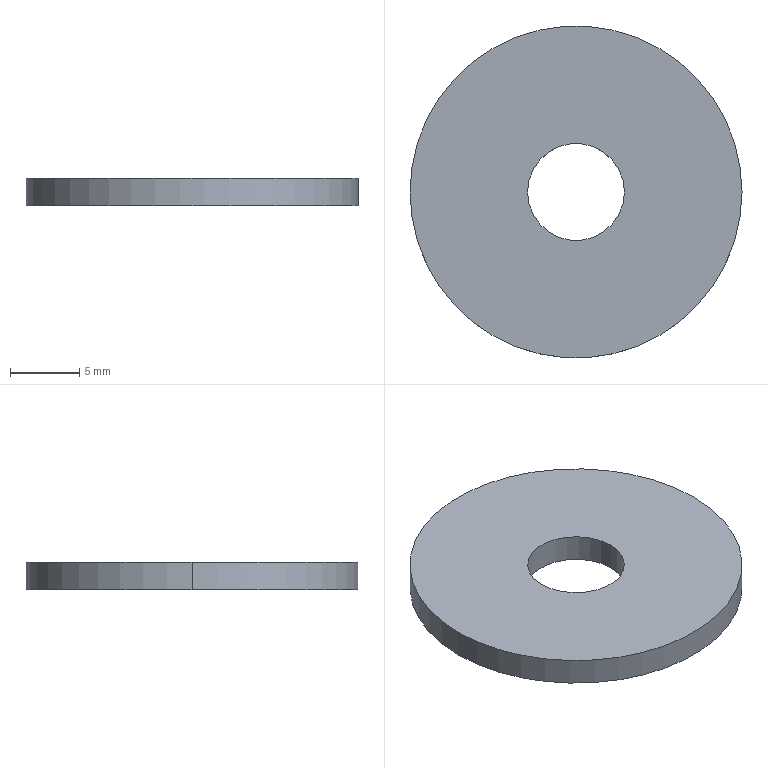Part | SolidWorks | features BaseBody 1 | 1 solid | 6 faces | box 24 x 24 x 2 mm | volume 827.81 mm3 | cylinder 4 | plane 2 | commonest cylinder face diameters 7 x2 24 x2
STEP:
#1=CARTESIAN_POINT('',(-12.,0.,2.));
#2=VERTEX_POINT('',#1);
#3=CARTESIAN_POINT('',(12.,0.,2.));
#4=VERTEX_POINT('',#3);
#5=CARTESIAN_POINT('',(0.,0.,2.));
#6=DIRECTION('',(0.,0.,-1.));
#7=DIRECTION('',(-1.,0.,0.));
#8=AXIS2_PLACEMENT_3D('',#5,#6,#7);
#9=CIRCLE('',#8,12.);
#10=EDGE_CURVE('',#2,#4,#9,.T.);
#11=ORIENTED_EDGE('',*,*,#10,.T.);
#12=CARTESIAN_POINT('',(12.,0.,0.));
#13=VERTEX_POINT('',#12);
#14=CARTESIAN_POINT('',(12.,0.,2.));
#15=DIRECTION('',(0.,0.,-1.));
#16=VECTOR('',#15,1000.);
#17=LINE('',#14,#16);
#18=EDGE_CURVE('',#4,#13,#17,.T.);
#19=ORIENTED_EDGE('',*,*,#18,.T.);
#20=CARTESIAN_POINT('',(-12.,0.,0.));
#21=VERTEX_POINT('',#20);
#22=CARTESIAN_POINT('',(0.,0.,0.));
#23=DIRECTION('',(0.,0.,1.));
#24=DIRECTION('',(-1.,0.,0.));
#25=AXIS2_PLACEMENT_3D('',#22,#23,#24);
#26=CIRCLE('',#25,12.);
#27=EDGE_CURVE('',#13,#21,#26,.T.);
#28=ORIENTED_EDGE('',*,*,#27,.T.);
#29=CARTESIAN_POINT('',(-12.,0.,2.));
#30=DIRECTION('',(0.,0.,-1.));
#31=VECTOR('',#30,1000.);
#32=LINE('',#29,#31);
#33=EDGE_CURVE('',#2,#21,#32,.T.);
#34=ORIENTED_EDGE('',*,*,#33,.F.);
#35=EDGE_LOOP('',(#11,#19,#28,#34));
#36=FACE_OUTER_BOUND('',#35,.T.);
#37=CARTESIAN_POINT('',(0.,0.,2.));
#38=DIRECTION('',(0.,0.,-1.));
#39=DIRECTION('',(-1.,0.,0.));
#40=AXIS2_PLACEMENT_3D('',#37,#38,#39);
#41=CYLINDRICAL_SURFACE('',#40,12.);
#42=ADVANCED_FACE('',(#36),#41,.T.);
#43=CARTESIAN_POINT('',(3.5,0.,0.));
#44=VERTEX_POINT('',#43);
#45=CARTESIAN_POINT('',(-3.5,0.,0.));
#46=VERTEX_POINT('',#45);
#47=CARTESIAN_POINT('',(0.,0.,0.));
#48=DIRECTION('',(0.,0.,-1.));
#49=DIRECTION('',(1.,0.,0.));
#50=AXIS2_PLACEMENT_3D('',#47,#48,#49);
#51=CIRCLE('',#50,3.5);
#52=EDGE_CURVE('',#44,#46,#51,.T.);
#53=ORIENTED_EDGE('',*,*,#52,.T.);
#54=CARTESIAN_POINT('',(-3.5,0.,2.));
#55=VERTEX_POINT('',#54);
#56=CARTESIAN_POINT('',(-3.5,0.,2.));
#57=DIRECTION('',(0.,0.,1.));
#58=VECTOR('',#57,1000.);
#59=LINE('',#56,#58);
#60=EDGE_CURVE('',#46,#55,#59,.T.);
#61=ORIENTED_EDGE('',*,*,#60,.T.);
#62=CARTESIAN_POINT('',(3.5,0.,2.));
#63=VERTEX_POINT('',#62);
#64=CARTESIAN_POINT('',(0.,0.,2.));
#65=DIRECTION('',(0.,0.,-1.));
#66=DIRECTION('',(1.,0.,0.));
#67=AXIS2_PLACEMENT_3D('',#64,#65,#66);
#68=CIRCLE('',#67,3.5);
#69=EDGE_CURVE('',#63,#55,#68,.T.);
#70=ORIENTED_EDGE('',*,*,#69,.F.);
#71=CARTESIAN_POINT('',(3.5,0.,2.));
#72=DIRECTION('',(0.,0.,1.));
#73=VECTOR('',#72,1000.);
#74=LINE('',#71,#73);
#75=EDGE_CURVE('',#44,#63,#74,.T.);
#76=ORIENTED_EDGE('',*,*,#75,.F.);
#77=EDGE_LOOP('',(#53,#61,#70,#76));
#78=FACE_OUTER_BOUND('',#77,.T.);
#79=CARTESIAN_POINT('',(0.,0.,2.));
#80=DIRECTION('',(0.,0.,1.));
#81=DIRECTION('',(1.,0.,0.));
#82=AXIS2_PLACEMENT_3D('',#79,#80,#81);
#83=CYLINDRICAL_SURFACE('',#82,3.5);
#84=ADVANCED_FACE('',(#78),#83,.F.);
#85=CARTESIAN_POINT('',(0.,0.,0.));
#86=DIRECTION('',(0.,0.,1.));
#87=DIRECTION('',(-1.,0.,0.));
#88=AXIS2_PLACEMENT_3D('',#85,#86,#87);
#89=CIRCLE('',#88,12.);
#90=EDGE_CURVE('',#21,#13,#89,.T.);
#91=ORIENTED_EDGE('',*,*,#90,.F.);
#92=ORIENTED_EDGE('',*,*,#27,.F.);
#93=EDGE_LOOP('',(#91,#92));
#94=FACE_OUTER_BOUND('',#93,.T.);
#95=ORIENTED_EDGE('',*,*,#52,.F.);
#96=CARTESIAN_POINT('',(0.,0.,0.));
#97=DIRECTION('',(0.,0.,-1.));
#98=DIRECTION('',(1.,0.,0.));
#99=AXIS2_PLACEMENT_3D('',#96,#97,#98);
#100=CIRCLE('',#99,3.5);
#101=EDGE_CURVE('',#46,#44,#100,.T.);
#102=ORIENTED_EDGE('',*,*,#101,.F.);
#103=EDGE_LOOP('',(#95,#102));
#104=FACE_BOUND('',#103,.T.);
#105=CARTESIAN_POINT('',(0.,0.,0.));
#106=DIRECTION('',(0.,0.,1.));
#107=DIRECTION('',(1.,0.,0.));
#108=AXIS2_PLACEMENT_3D('',#105,#106,#107);
#109=PLANE('',#108);
#110=ADVANCED_FACE('',(#94,#104),#109,.F.);
#111=ORIENTED_EDGE('',*,*,#18,.F.);
#112=CARTESIAN_POINT('',(0.,0.,2.));
#113=DIRECTION('',(0.,0.,-1.));
#114=DIRECTION('',(-1.,0.,0.));
#115=AXIS2_PLACEMENT_3D('',#112,#113,#114);
#116=CIRCLE('',#115,12.);
#117=EDGE_CURVE('',#4,#2,#116,.T.);
#118=ORIENTED_EDGE('',*,*,#117,.T.);
#119=ORIENTED_EDGE('',*,*,#33,.T.);
#120=ORIENTED_EDGE('',*,*,#90,.T.);
#121=EDGE_LOOP('',(#111,#118,#119,#120));
#122=FACE_OUTER_BOUND('',#121,.T.);
#123=CARTESIAN_POINT('',(0.,0.,2.));
#124=DIRECTION('',(0.,0.,-1.));
#125=DIRECTION('',(-1.,0.,0.));
#126=AXIS2_PLACEMENT_3D('',#123,#124,#125);
#127=CYLINDRICAL_SURFACE('',#126,12.);
#128=ADVANCED_FACE('',(#122),#127,.T.);
#129=ORIENTED_EDGE('',*,*,#60,.F.);
#130=ORIENTED_EDGE('',*,*,#101,.T.);
#131=ORIENTED_EDGE('',*,*,#75,.T.);
#132=CARTESIAN_POINT('',(0.,0.,2.));
#133=DIRECTION('',(0.,0.,-1.));
#134=DIRECTION('',(1.,0.,0.));
#135=AXIS2_PLACEMENT_3D('',#132,#133,#134);
#136=CIRCLE('',#135,3.5);
#137=EDGE_CURVE('',#55,#63,#136,.T.);
#138=ORIENTED_EDGE('',*,*,#137,.F.);
#139=EDGE_LOOP('',(#129,#130,#131,#138));
#140=FACE_OUTER_BOUND('',#139,.T.);
#141=CARTESIAN_POINT('',(0.,0.,2.));
#142=DIRECTION('',(0.,0.,1.));
#143=DIRECTION('',(1.,0.,0.));
#144=AXIS2_PLACEMENT_3D('',#141,#142,#143);
#145=CYLINDRICAL_SURFACE('',#144,3.5);
#146=ADVANCED_FACE('',(#140),#145,.F.);
#147=ORIENTED_EDGE('',*,*,#10,.F.);
#148=ORIENTED_EDGE('',*,*,#117,.F.);
#149=EDGE_LOOP('',(#147,#148));
#150=FACE_OUTER_BOUND('',#149,.T.);
#151=ORIENTED_EDGE('',*,*,#69,.T.);
#152=ORIENTED_EDGE('',*,*,#137,.T.);
#153=EDGE_LOOP('',(#151,#152));
#154=FACE_BOUND('',#153,.T.);
#155=CARTESIAN_POINT('',(0.,0.,2.));
#156=DIRECTION('',(0.,0.,1.));
#157=DIRECTION('',(1.,0.,0.));
#158=AXIS2_PLACEMENT_3D('',#155,#156,#157);
#159=PLANE('',#158);
#160=ADVANCED_FACE('',(#150,#154),#159,.T.);
#161=CLOSED_SHELL('',(#42,#84,#110,#128,#146,#160));
#162=MANIFOLD_SOLID_BREP('',#161);
#163=CARTESIAN_POINT('',(0.,0.,0.));
#164=DIRECTION('',(0.,0.,1.));
#165=DIRECTION('',(1.,0.,0.));
#166=AXIS2_PLACEMENT_3D('',#163,#164,#165);
#167=(LENGTH_UNIT()NAMED_UNIT(*)SI_UNIT(.MILLI.,.METRE.));
#168=UNCERTAINTY_MEASURE_WITH_UNIT(LENGTH_MEASURE(0.00001),#167,'','');
#169=(NAMED_UNIT(*)PLANE_ANGLE_UNIT()SI_UNIT($,.RADIAN.));
#170=(NAMED_UNIT(*)SI_UNIT($,.STERADIAN.)SOLID_ANGLE_UNIT());
#171=(GEOMETRIC_REPRESENTATION_CONTEXT(3)GLOBAL_UNCERTAINTY_ASSIGNED_CONTEXT((#168))GLOBAL_UNIT_ASSIGNED_CONTEXT((#167,#169,#170))REPRESENTATION_CONTEXT('',''));
#172=ADVANCED_BREP_SHAPE_REPRESENTATION('',(#162,#166),#171);